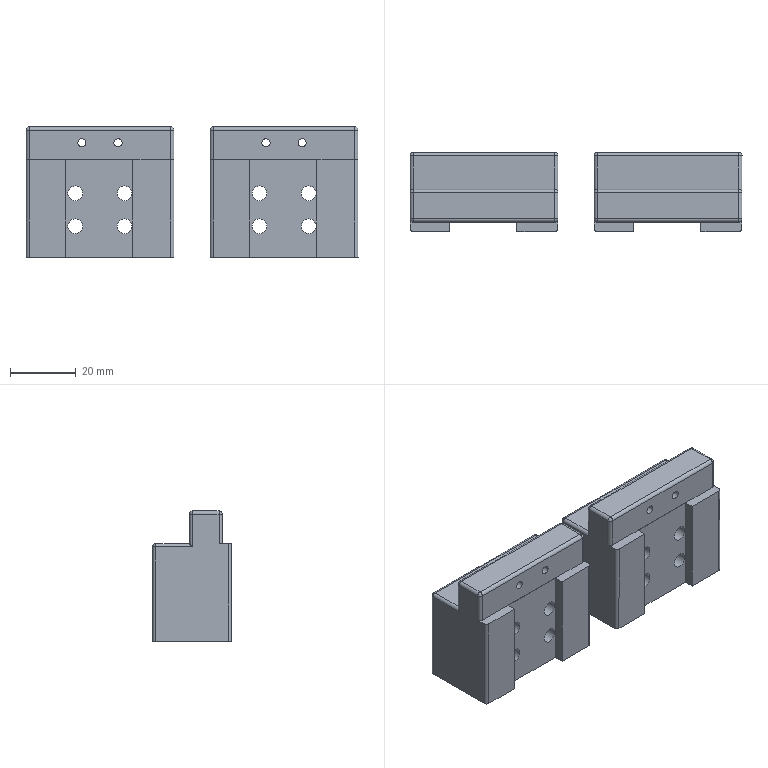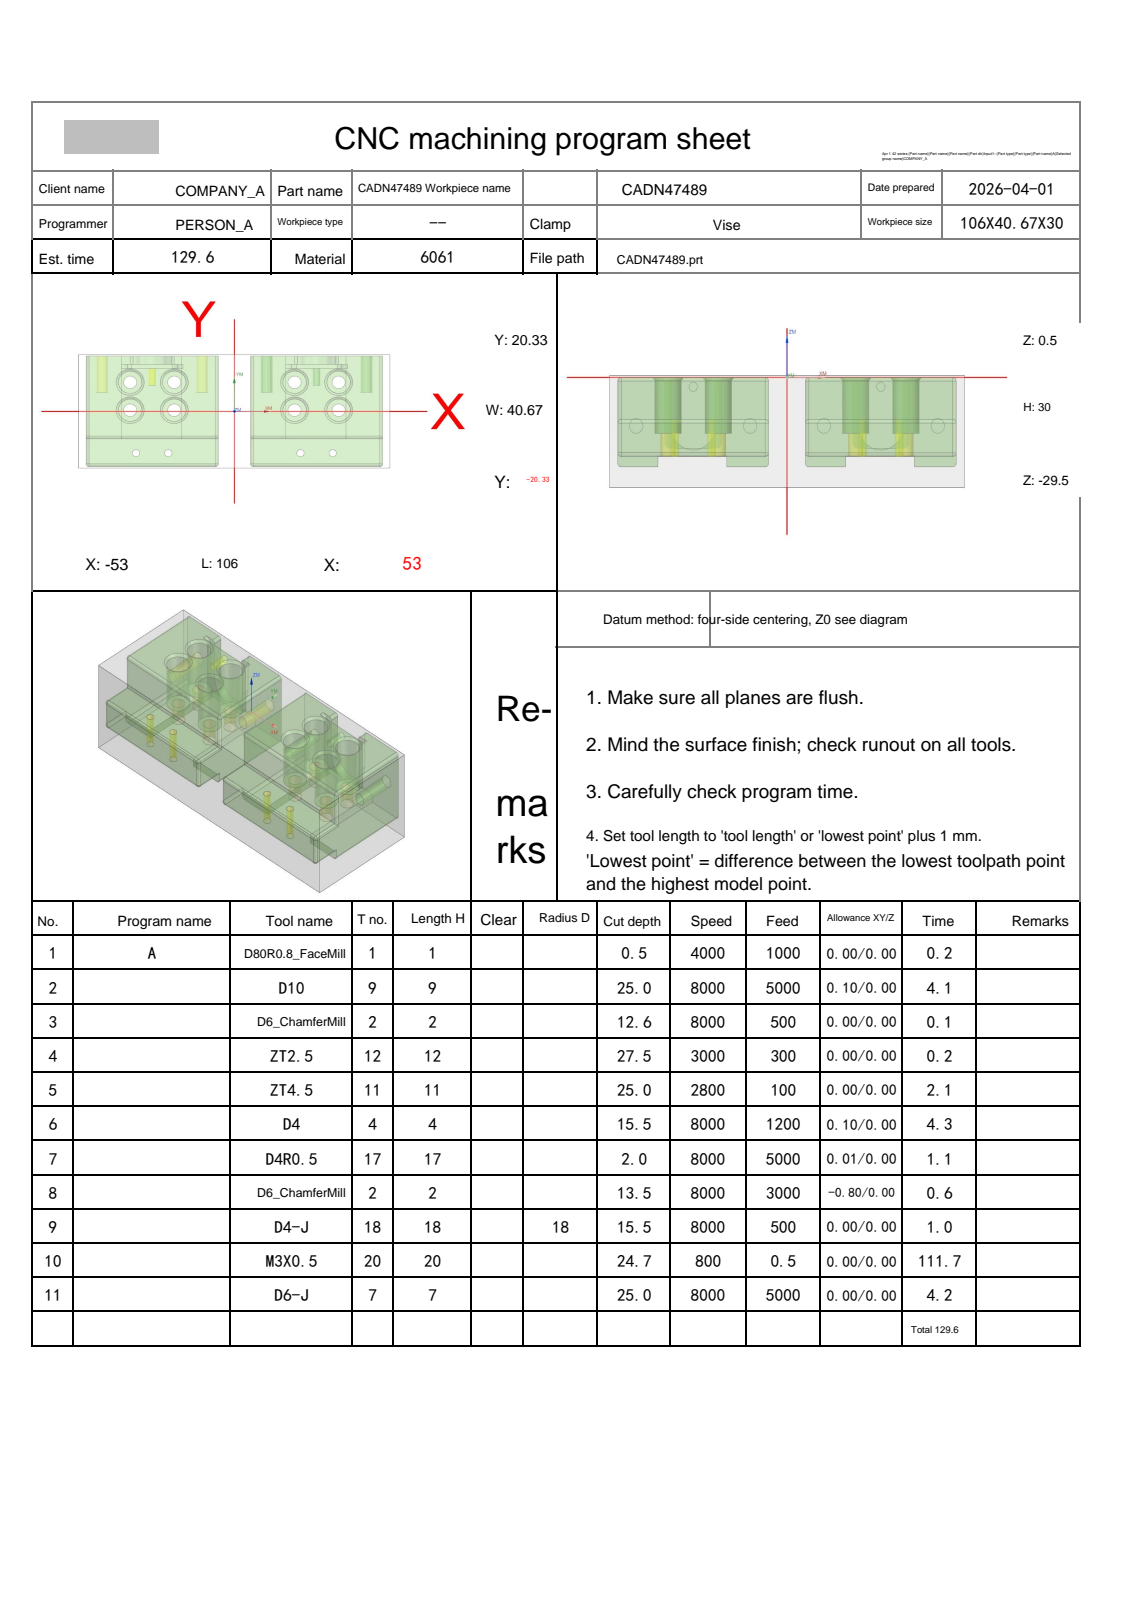NC program | NX | posted by the shop | part box 101.001 x 24.001 x 39.667 mm
Lines 1 to 2473 of 28944, first 1640 of 2471 lines:
%
O0001
(Machine time: 235.25 MIN)
(===Total Tool:10===)
(T1=D80R0.8 face mill D=80.  R=0.8  D-  H01 Z=0.    )
(T9=D10     D=10.  R=0.   D-  H09 Z=-24.5 )
(T2=D6_ChamferMill   D=6.   R=0.   D-  H02 Z=-13.01)
(T12=ZT2.5  D=2.5  DR_a=118 D-  H12 Z=-26.97)
(T11=ZT4.5  D=4.5  DR_a=118 D-  H11 Z=-24.45)
(T4=D4      D=4.   R=0.   D-  H04 Z=-15.  )
(T17=D4R0.5 D=4.   R=0.5  D-  H17 Z=-1.5  )
(T18=D4-J   D=4.   R=0.   D18 H18 Z=-15.  )
(T20=M3X0.5 D=2.5  DR_a=180 D-  H20 Z=-24.22)
(T7=D6-J    D=6.   R=0.   D7  H07 Z=-24.5 )
G80 G90 G17 G49 G40
G91 G28 Z0
M01
N1 T01 M06
(D80R0.8 face mill  D=80. R=0.8 H=01 ce=0.00 di=0.00)
G00 G90 G54 X95.501 Y0.0 M03 S4000
G43 H01 Z20.
M08
Z2.
G01 Z0.0 F1000.
X90.501
X-90.5
X-95.5
Z2.
G00 Z20.
G91 G28 Z0.0
M05
M09
G91 G28 Z0.0
M01
N2 T09 M06
(D10  D=10. R=0. H=09 ce=0.10 di=0.00)
G00 G90 G54 X-52.062 Y-24.399 M03 S8000
G43 H09 Z20.
M08
Z.5
G01 X-53.212 Y-23.713 Z.495 F5000.
X-54.216 Y-22.755 Z.489
X-54.985 Y-21.576 Z.484
X-55.467 Y-20.254 Z.478
X-55.6 Y-19.136 Z.474
Y19.833 Z.322
G02 X-50.5 Y24.933 Z.291 I5.1 J0.0
G01 X-6.498 Z.12
X-5.496 Y24.932 Z.116
G02 X-.4 Y19.832 Z.084 I-.004 J-5.1
G01 Y-18.833 Z-.066
G02 X-6.5 Y-24.932 Z-.103 I-6.1 J.001
G01 X-49.741 Z-.272
X-50.776 Y-24.828 Z-.276
X-52.05 Y-24.406 Z-.281
X-53.212 Y-23.713 Z-.286
X-54.216 Y-22.755 Z-.292
X-54.985 Y-21.576 Z-.297
X-55.467 Y-20.254 Z-.303
X-55.6 Y-19.136 Z-.307
Y19.833 Z-.459
G02 X-50.5 Y24.933 Z-.49 I5.1 J0.0
G01 X-6.498 Z-.662
X-5.496 Y24.932 Z-.666
G02 X-.4 Y19.832 Z-.697 I-.004 J-5.1
G01 Y-18.833 Z-.847
G02 X-6.5 Y-24.932 Z-.885 I-6.1 J.001
G01 X-49.741 Z-1.053
X-50.776 Y-24.828 Z-1.057
X-52.05 Y-24.406 Z-1.062
X-53.212 Y-23.713 Z-1.068
X-54.216 Y-22.755 Z-1.073
X-54.985 Y-21.576 Z-1.079
X-55.467 Y-20.254 Z-1.084
X-55.6 Y-19.136 Z-1.088
Y19.833 Z-1.24
G02 X-50.5 Y24.933 Z-1.272 I5.1 J0.0
G01 X-6.498 Z-1.443
X-5.496 Y24.932 Z-1.447
G02 X-.4 Y19.832 Z-1.478 I-.004 J-5.1
G01 Y-18.833 Z-1.629
G02 X-6.5 Y-24.932 Z-1.666 I-6.1 J.001
G01 X-49.741 Z-1.834
X-50.776 Y-24.828 Z-1.838
X-52.05 Y-24.406 Z-1.844
X-53.212 Y-23.713 Z-1.849
X-54.216 Y-22.755 Z-1.854
X-54.985 Y-21.576 Z-1.86
X-55.467 Y-20.254 Z-1.865
X-55.6 Y-19.136 Z-1.87
Y19.833 Z-2.022
G02 X-50.5 Y24.933 Z-2.053 I5.1 J0.0
G01 X-6.498 Z-2.224
X-5.496 Y24.932 Z-2.228
G02 X-.4 Y19.832 Z-2.259 I-.004 J-5.1
G01 Y-18.833 Z-2.41
G02 X-6.5 Y-24.932 Z-2.447 I-6.1 J.001
G01 X-49.741 Z-2.616
X-50.776 Y-24.828 Z-2.62
X-52.05 Y-24.406 Z-2.625
X-53.212 Y-23.713 Z-2.63
X-54.216 Y-22.755 Z-2.636
X-54.985 Y-21.576 Z-2.641
X-55.467 Y-20.254 Z-2.647
X-55.6 Y-19.136 Z-2.651
Y19.833 Z-2.803
G02 X-50.5 Y24.933 Z-2.834 I5.1 J0.0
G01 X-6.498 Z-3.005
X-5.496 Y24.932 Z-3.009
G02 X-.4 Y19.832 Z-3.041 I-.004 J-5.1
G01 Y-18.833 Z-3.191
G02 X-6.5 Y-24.932 Z-3.228 I-6.1 J.001
G01 X-49.741 Z-3.397
X-50.776 Y-24.828 Z-3.401
X-52.05 Y-24.406 Z-3.406
X-53.212 Y-23.713 Z-3.411
X-54.216 Y-22.755 Z-3.417
X-54.985 Y-21.576 Z-3.422
X-55.467 Y-20.254 Z-3.428
X-55.6 Y-19.136 Z-3.432
Y19.833 Z-3.584
G02 X-50.5 Y24.933 Z-3.615 I5.1 J0.0
G01 X-6.498 Z-3.787
X-5.496 Y24.932 Z-3.791
G02 X-.4 Y19.832 Z-3.822 I-.004 J-5.1
G01 Y-18.833 Z-3.972
G02 X-6.5 Y-24.932 Z-4.01 I-6.1 J.001
G01 X-49.741 Z-4.178
X-50.776 Y-24.828 Z-4.182
X-52.05 Y-24.406 Z-4.187
X-53.212 Y-23.713 Z-4.193
X-54.216 Y-22.755 Z-4.198
X-54.985 Y-21.576 Z-4.204
X-55.467 Y-20.254 Z-4.209
X-55.6 Y-19.136 Z-4.214
Y19.833 Z-4.365
G02 X-50.5 Y24.933 Z-4.397 I5.1 J0.0
G01 X-6.498 Z-4.568
X-5.496 Y24.932 Z-4.572
G02 X-.4 Y19.832 Z-4.603 I-.004 J-5.1
G01 Y-18.833 Z-4.754
G02 X-6.5 Y-24.932 Z-4.791 I-6.1 J.001
G01 X-49.741 Z-4.959
X-50.776 Y-24.828 Z-4.964
X-52.05 Y-24.406 Z-4.969
X-53.212 Y-23.713 Z-4.974
X-54.216 Y-22.755 Z-4.979
X-54.985 Y-21.576 Z-4.985
X-55.467 Y-20.254 Z-4.99
X-55.6 Y-19.136 Z-4.995
Y19.833 Z-5.147
G02 X-50.5 Y24.933 Z-5.178 I5.1 J0.0
G01 X-6.498 Z-5.349
X-5.496 Y24.932 Z-5.353
G02 X-.4 Y19.832 Z-5.384 I-.004 J-5.1
G01 Y-18.833 Z-5.535
G02 X-6.5 Y-24.932 Z-5.572 I-6.1 J.001
G01 X-49.741 Z-5.741
X-50.776 Y-24.828 Z-5.745
X-52.05 Y-24.406 Z-5.75
X-53.212 Y-23.713 Z-5.755
X-54.216 Y-22.755 Z-5.761
X-54.985 Y-21.576 Z-5.766
X-55.467 Y-20.254 Z-5.772
X-55.6 Y-19.136 Z-5.776
Y19.833 Z-5.928
G02 X-50.5 Y24.933 Z-5.959 I5.1 J0.0
G01 X-6.498 Z-6.13
X-5.496 Y24.932 Z-6.134
G02 X-.4 Y19.832 Z-6.166 I-.004 J-5.1
G01 Y-18.833 Z-6.316
G02 X-6.5 Y-24.932 Z-6.354 I-6.1 J.001
G01 X-49.741 Z-6.522
X-50.776 Y-24.828 Z-6.526
X-52.05 Y-24.406 Z-6.531
X-53.212 Y-23.713 Z-6.537
X-54.216 Y-22.755 Z-6.542
X-54.985 Y-21.576 Z-6.547
X-55.467 Y-20.254 Z-6.553
X-55.6 Y-19.136 Z-6.557
Y19.833 Z-6.709
G02 X-50.5 Y24.933 Z-6.74 I5.1 J0.0
G01 X-6.498 Z-6.912
X-5.496 Y24.932 Z-6.916
G02 X-.4 Y19.832 Z-6.947 I-.004 J-5.1
G01 Y-18.833 Z-7.097
G02 X-6.5 Y-24.932 Z-7.135 I-6.1 J.001
G01 X-49.741 Z-7.303
X-50.776 Y-24.828 Z-7.307
X-52.05 Y-24.406 Z-7.313
X-53.212 Y-23.713 Z-7.318
X-54.216 Y-22.755 Z-7.323
X-54.985 Y-21.576 Z-7.329
X-55.467 Y-20.254 Z-7.334
X-55.6 Y-19.136 Z-7.339
Y19.833 Z-7.49
G02 X-50.5 Y24.933 Z-7.522 I5.1 J0.0
G01 X-6.498 Z-7.693
X-5.496 Y24.932 Z-7.697
G02 X-.4 Y19.832 Z-7.728 I-.004 J-5.1
G01 Y-18.833 Z-7.879
G02 X-6.5 Y-24.932 Z-7.916 I-6.1 J.001
G01 X-49.741 Z-8.084
X-50.776 Y-24.828 Z-8.089
X-52.05 Y-24.406 Z-8.094
X-53.212 Y-23.713 Z-8.099
X-54.216 Y-22.755 Z-8.104
X-54.985 Y-21.576 Z-8.11
X-55.467 Y-20.254 Z-8.115
X-55.6 Y-19.136 Z-8.12
Y19.833 Z-8.272
G02 X-50.5 Y24.933 Z-8.303 I5.1 J0.0
G01 X-6.498 Z-8.474
X-5.496 Y24.932 Z-8.478
G02 X-.4 Y19.832 Z-8.509 I-.004 J-5.1
G01 Y-18.833 Z-8.66
G02 X-6.5 Y-24.932 Z-8.697 I-6.1 J.001
G01 X-49.741 Z-8.866
X-50.776 Y-24.828 Z-8.87
X-52.05 Y-24.406 Z-8.875
X-53.212 Y-23.713 Z-8.88
X-54.216 Y-22.755 Z-8.886
X-54.985 Y-21.576 Z-8.891
X-55.467 Y-20.254 Z-8.897
X-55.6 Y-19.136 Z-8.901
Y19.833 Z-9.053
G02 X-50.5 Y24.933 Z-9.084 I5.1 J0.0
G01 X-6.498 Z-9.255
X-5.496 Y24.932 Z-9.259
G02 X-.4 Y19.832 Z-9.291 I-.004 J-5.1
G01 Y-18.833 Z-9.441
G02 X-6.5 Y-24.932 Z-9.479 I-6.1 J.001
G01 X-49.741 Z-9.647
X-50.776 Y-24.828 Z-9.651
X-52.05 Y-24.406 Z-9.656
X-53.212 Y-23.713 Z-9.662
X-54.216 Y-22.755 Z-9.667
X-54.985 Y-21.576 Z-9.672
X-55.467 Y-20.254 Z-9.678
X-55.6 Y-19.136 Z-9.682
Y19.833 Z-9.834
G02 X-50.5 Y24.933 Z-9.865 I5.1 J0.0
G01 X-6.498 Z-10.037
X-5.496 Y24.932 Z-10.041
G02 X-.4 Y19.832 Z-10.072 I-.004 J-5.1
G01 Y-18.833 Z-10.222
G02 X-6.5 Y-24.932 Z-10.26 I-6.1 J.001
G01 X-49.741 Z-10.428
X-50.776 Y-24.828 Z-10.432
X-52.05 Y-24.406 Z-10.438
X-53.212 Y-23.713 Z-10.443
X-54.216 Y-22.755 Z-10.448
X-54.985 Y-21.576 Z-10.454
X-55.467 Y-20.254 Z-10.459
X-55.6 Y-19.136 Z-10.464
Y19.833 Z-10.615
G02 X-50.5 Y24.933 Z-10.647 I5.1 J0.0
G01 X-6.498 Z-10.818
X-5.496 Y24.932 Z-10.822
G02 X-.4 Y19.832 Z-10.853 I-.004 J-5.1
G01 Y-18.833 Z-11.004
G02 X-6.5 Y-24.932 Z-11.041 I-6.1 J.001
G01 X-49.741 Z-11.21
X-50.776 Y-24.828 Z-11.214
X-52.05 Y-24.406 Z-11.219
X-53.212 Y-23.713 Z-11.224
X-54.216 Y-22.755 Z-11.229
X-54.985 Y-21.576 Z-11.235
X-55.467 Y-20.254 Z-11.24
X-55.6 Y-19.136 Z-11.245
Y19.833 Z-11.397
G02 X-50.5 Y24.933 Z-11.428 I5.1 J0.0
G01 X-6.498 Z-11.599
X-5.496 Y24.932 Z-11.603
G02 X-.4 Y19.832 Z-11.634 I-.004 J-5.1
G01 Y-18.833 Z-11.785
G02 X-6.5 Y-24.932 Z-11.822 I-6.1 J.001
G01 X-49.741 Z-11.991
X-50.776 Y-24.828 Z-11.995
X-52.05 Y-24.406 Z-12.
X-53.212 Y-23.713 Z-12.005
X-54.216 Y-22.755 Z-12.011
X-54.985 Y-21.576 Z-12.016
X-55.467 Y-20.254 Z-12.022
X-55.6 Y-19.136 Z-12.026
Y19.833 Z-12.178
G02 X-50.5 Y24.933 Z-12.209 I5.1 J0.0
G01 X-6.498 Z-12.381
X-5.496 Y24.932 Z-12.384
G02 X-.4 Y19.832 Z-12.416 I-.004 J-5.1
G01 Y-18.833 Z-12.566
G02 X-6.5 Y-24.932 Z-12.604 I-6.1 J.001
G01 X-49.741 Z-12.772
X-50.776 Y-24.828 Z-12.776
X-52.05 Y-24.406 Z-12.781
X-53.212 Y-23.713 Z-12.787
X-54.216 Y-22.755 Z-12.792
X-54.985 Y-21.576 Z-12.797
X-55.467 Y-20.254 Z-12.803
X-55.6 Y-19.136 Z-12.807
Y19.833 Z-12.959
G02 X-50.5 Y24.933 Z-12.99 I5.1 J0.0
G01 X-6.498 Z-13.162
X-5.496 Y24.932 Z-13.166
G02 X-.4 Y19.832 Z-13.197 I-.004 J-5.1
G01 Y-18.833 Z-13.347
G02 X-6.5 Y-24.932 Z-13.385 I-6.1 J.001
G01 X-49.741 Z-13.553
X-50.776 Y-24.828 Z-13.557
X-52.05 Y-24.406 Z-13.563
X-53.212 Y-23.713 Z-13.568
X-54.216 Y-22.755 Z-13.573
X-54.985 Y-21.576 Z-13.579
X-55.467 Y-20.254 Z-13.584
X-55.6 Y-19.136 Z-13.589
Y19.833 Z-13.74
G02 X-50.5 Y24.933 Z-13.772 I5.1 J0.0
G01 X-6.498 Z-13.943
X-5.496 Y24.932 Z-13.947
G02 X-.4 Y19.832 Z-13.978 I-.004 J-5.1
G01 Y-18.833 Z-14.129
G02 X-6.5 Y-24.932 Z-14.166 I-6.1 J.001
G01 X-49.741 Z-14.335
X-50.776 Y-24.828 Z-14.339
X-52.05 Y-24.406 Z-14.344
X-53.212 Y-23.713 Z-14.349
X-54.216 Y-22.755 Z-14.354
X-54.985 Y-21.576 Z-14.36
X-55.467 Y-20.254 Z-14.365
X-55.6 Y-19.136 Z-14.37
Y19.833 Z-14.522
G02 X-50.5 Y24.933 Z-14.553 I5.1 J0.0
G01 X-6.498 Z-14.724
X-5.496 Y24.932 Z-14.728
G02 X-.4 Y19.832 Z-14.759 I-.004 J-5.1
G01 Y-18.833 Z-14.91
G02 X-6.5 Y-24.932 Z-14.947 I-6.1 J.001
G01 X-49.741 Z-15.116
X-50.776 Y-24.828 Z-15.12
X-52.05 Y-24.406 Z-15.125
X-53.212 Y-23.713 Z-15.13
X-54.216 Y-22.755 Z-15.136
X-54.985 Y-21.576 Z-15.141
X-55.467 Y-20.254 Z-15.147
X-55.6 Y-19.136 Z-15.151
Y19.833 Z-15.303
G02 X-50.5 Y24.933 Z-15.334 I5.1 J0.0
G01 X-6.498 Z-15.506
X-5.496 Y24.932 Z-15.509
G02 X-.4 Y19.832 Z-15.541 I-.004 J-5.1
G01 Y-18.833 Z-15.691
G02 X-6.5 Y-24.932 Z-15.729 I-6.1 J.001
G01 X-49.741 Z-15.897
X-50.776 Y-24.828 Z-15.901
X-52.05 Y-24.406 Z-15.906
X-53.212 Y-23.713 Z-15.912
X-54.216 Y-22.755 Z-15.917
X-54.985 Y-21.576 Z-15.922
X-55.467 Y-20.254 Z-15.928
X-55.6 Y-19.136 Z-15.932
Y19.833 Z-16.084
G02 X-50.5 Y24.933 Z-16.115 I5.1 J0.0
G01 X-6.498 Z-16.287
X-5.496 Y24.932 Z-16.291
G02 X-.4 Y19.832 Z-16.322 I-.004 J-5.1
G01 Y-18.833 Z-16.473
G02 X-6.5 Y-24.932 Z-16.51 I-6.1 J.001
G01 X-49.741 Z-16.678
X-50.776 Y-24.828 Z-16.682
X-52.05 Y-24.406 Z-16.688
X-53.212 Y-23.713 Z-16.693
X-54.216 Y-22.755 Z-16.698
X-54.985 Y-21.576 Z-16.704
X-55.467 Y-20.254 Z-16.709
X-55.6 Y-19.136 Z-16.714
Y19.833 Z-16.865
G02 X-50.5 Y24.933 Z-16.897 I5.1 J0.0
G01 X-6.498 Z-17.068
X-5.496 Y24.932 Z-17.072
G02 X-.4 Y19.832 Z-17.103 I-.004 J-5.1
G01 Y-18.833 Z-17.254
G02 X-6.5 Y-24.932 Z-17.291 I-6.1 J.001
G01 X-49.741 Z-17.46
X-50.776 Y-24.828 Z-17.464
X-52.05 Y-24.406 Z-17.469
X-53.212 Y-23.713 Z-17.474
X-54.216 Y-22.755 Z-17.48
X-54.985 Y-21.576 Z-17.485
X-55.467 Y-20.254 Z-17.49
X-55.6 Y-19.136 Z-17.495
Y19.833 Z-17.647
G02 X-50.5 Y24.933 Z-17.678 I5.1 J0.0
G01 X-6.498 Z-17.849
X-5.496 Y24.932 Z-17.853
G02 X-.4 Y19.832 Z-17.884 I-.004 J-5.1
G01 Y-18.833 Z-18.035
G02 X-6.5 Y-24.932 Z-18.072 I-6.1 J.001
G01 X-49.741 Z-18.241
X-50.776 Y-24.828 Z-18.245
X-52.05 Y-24.406 Z-18.25
X-53.212 Y-23.713 Z-18.255
X-54.216 Y-22.755 Z-18.261
X-54.985 Y-21.576 Z-18.266
X-55.467 Y-20.254 Z-18.272
X-55.6 Y-19.136 Z-18.276
Y19.833 Z-18.428
G02 X-50.5 Y24.933 Z-18.459 I5.1 J0.0
G01 X-6.498 Z-18.631
X-5.496 Y24.932 Z-18.634
G02 X-.4 Y19.832 Z-18.666 I-.004 J-5.1
G01 Y-18.833 Z-18.816
G02 X-6.5 Y-24.932 Z-18.854 I-6.1 J.001
G01 X-49.741 Z-19.022
X-50.776 Y-24.828 Z-19.026
X-52.05 Y-24.406 Z-19.031
X-53.212 Y-23.713 Z-19.037
X-54.216 Y-22.755 Z-19.042
X-54.985 Y-21.576 Z-19.047
X-55.467 Y-20.254 Z-19.053
X-55.6 Y-19.136 Z-19.057
Y19.833 Z-19.209
G02 X-50.5 Y24.933 Z-19.24 I5.1 J0.0
G01 X-6.498 Z-19.412
X-5.496 Y24.932 Z-19.416
G02 X-.4 Y19.832 Z-19.447 I-.004 J-5.1
G01 Y-18.833 Z-19.598
G02 X-6.5 Y-24.932 Z-19.635 I-6.1 J.001
G01 X-49.741 Z-19.803
X-50.776 Y-24.828 Z-19.807
X-52.05 Y-24.406 Z-19.813
X-53.212 Y-23.713 Z-19.818
X-54.216 Y-22.755 Z-19.823
X-54.985 Y-21.576 Z-19.829
X-55.467 Y-20.254 Z-19.834
X-55.6 Y-19.136 Z-19.839
Y19.833 Z-19.99
G02 X-50.5 Y24.933 Z-20.022 I5.1 J0.0
G01 X-6.498 Z-20.193
X-5.496 Y24.932 Z-20.197
G02 X-.4 Y19.832 Z-20.228 I-.004 J-5.1
G01 Y-18.833 Z-20.379
G02 X-6.5 Y-24.932 Z-20.416 I-6.1 J.001
G01 X-49.741 Z-20.585
X-50.776 Y-24.828 Z-20.589
X-52.05 Y-24.406 Z-20.594
X-53.212 Y-23.713 Z-20.599
X-54.216 Y-22.755 Z-20.605
X-54.985 Y-21.576 Z-20.61
X-55.467 Y-20.254 Z-20.615
X-55.6 Y-19.136 Z-20.62
Y19.833 Z-20.772
G02 X-50.5 Y24.933 Z-20.803 I5.1 J0.0
G01 X-6.498 Z-20.974
X-5.496 Y24.932 Z-20.978
G02 X-.4 Y19.832 Z-21.009 I-.004 J-5.1
G01 Y-18.833 Z-21.16
G02 X-6.5 Y-24.932 Z-21.197 I-6.1 J.001
G01 X-49.741 Z-21.366
X-50.776 Y-24.828 Z-21.37
X-52.05 Y-24.406 Z-21.375
X-53.212 Y-23.713 Z-21.38
X-54.216 Y-22.755 Z-21.386
X-54.985 Y-21.576 Z-21.391
X-55.467 Y-20.254 Z-21.397
X-55.6 Y-19.136 Z-21.401
Y19.833 Z-21.553
G02 X-50.5 Y24.933 Z-21.584 I5.1 J0.0
G01 X-6.498 Z-21.756
X-5.496 Y24.932 Z-21.759
G02 X-.4 Y19.832 Z-21.791 I-.004 J-5.1
G01 Y-18.833 Z-21.941
G02 X-6.5 Y-24.932 Z-21.979 I-6.1 J.001
G01 X-49.741 Z-22.147
X-50.776 Y-24.828 Z-22.151
X-52.05 Y-24.406 Z-22.156
X-53.212 Y-23.713 Z-22.162
X-54.216 Y-22.755 Z-22.167
X-54.985 Y-21.576 Z-22.173
X-55.467 Y-20.254 Z-22.178
X-55.6 Y-19.136 Z-22.182
Y19.833 Z-22.334
G02 X-50.5 Y24.933 Z-22.365 I5.1 J0.0
G01 X-6.498 Z-22.537
X-5.496 Y24.932 Z-22.541
G02 X-.4 Y19.832 Z-22.572 I-.004 J-5.1
G01 Y-18.833 Z-22.723
G02 X-6.5 Y-24.932 Z-22.76 I-6.1 J.001
G01 X-49.741 Z-22.928
X-50.776 Y-24.828 Z-22.932
X-52.05 Y-24.406 Z-22.938
X-53.212 Y-23.713 Z-22.943
X-54.216 Y-22.755 Z-22.948
X-54.985 Y-21.576 Z-22.954
X-55.467 Y-20.254 Z-22.959
X-55.6 Y-19.136 Z-22.964
Y19.833 Z-23.115
G02 X-50.5 Y24.933 Z-23.147 I5.1 J0.0
G01 X-6.498 Z-23.318
X-5.496 Y24.932 Z-23.322
G02 X-.4 Y19.832 Z-23.353 I-.004 J-5.1
G01 Y-18.833 Z-23.504
G02 X-6.5 Y-24.932 Z-23.541 I-6.1 J.001
G01 X-49.741 Z-23.71
X-50.776 Y-24.828 Z-23.714
X-52.05 Y-24.406 Z-23.719
X-53.212 Y-23.713 Z-23.724
X-54.216 Y-22.755 Z-23.73
X-54.985 Y-21.576 Z-23.735
X-55.467 Y-20.254 Z-23.741
X-55.6 Y-19.136 Z-23.745
Y19.833 Z-23.897
G02 X-50.5 Y24.933 Z-23.928 I5.1 J0.0
G01 X-6.498 Z-24.099
X-5.496 Y24.932 Z-24.103
G02 X-.4 Y19.832 Z-24.134 I-.004 J-5.1
G01 Y-18.833 Z-24.285
G02 X-6.5 Y-24.932 Z-24.322 I-6.1 J.001
G01 X-49.741 Z-24.491
X-50.776 Y-24.828 Z-24.495
X-52.05 Y-24.406 Z-24.5
X-53.212 Y-23.713
X-54.216 Y-22.755
X-54.985 Y-21.576
X-55.467 Y-20.254
X-55.6 Y-19.136
Y19.833
G02 X-50.5 Y24.933 I5.1 J0.0
G01 X-6.498
X-5.496 Y24.932
G02 X-.4 Y19.832 I-.004 J-5.1
G01 Y-18.833
G02 X-6.5 Y-24.932 I-6.1 J.001
G01 X-49.741
X-50.776 Y-24.828
X-52.05 Y-24.406
X-52.062 Y-24.399
X-52.491 Y-24.143
Z-23.5
G00 Z20.
X3.938 Y-24.4
Z.5
G01 X2.788 Y-23.714 Z.495
X1.784 Y-22.756 Z.489
X1.015 Y-21.577 Z.484
X.533 Y-20.255 Z.478
X.4 Y-19.137 Z.474
Y19.832 Z.322
G02 X5.5 Y24.932 Z.291 I5.1 J0.0
G01 X49.502 Z.12
X50.504 Y24.931 Z.116
G02 X55.6 Y19.831 Z.084 I-.004 J-5.1
G01 Y-18.834 Z-.066
G02 X49.5 Y-24.933 Z-.103 I-6.1 J.001
G01 X6.259 Z-.272
X5.224 Y-24.829 Z-.276
X3.95 Y-24.406 Z-.281
X2.788 Y-23.714 Z-.286
X1.784 Y-22.756 Z-.292
X1.015 Y-21.577 Z-.297
X.533 Y-20.255 Z-.303
X.4 Y-19.137 Z-.307
Y19.832 Z-.459
G02 X5.5 Y24.932 Z-.49 I5.1 J0.0
G01 X49.502 Z-.662
X50.504 Y24.931 Z-.666
G02 X55.6 Y19.831 Z-.697 I-.004 J-5.1
G01 Y-18.834 Z-.847
G02 X49.5 Y-24.933 Z-.885 I-6.1 J.001
G01 X6.259 Z-1.053
X5.224 Y-24.829 Z-1.057
X3.95 Y-24.406 Z-1.062
X2.788 Y-23.714 Z-1.068
X1.784 Y-22.756 Z-1.073
X1.015 Y-21.577 Z-1.079
X.533 Y-20.255 Z-1.084
X.4 Y-19.137 Z-1.088
Y19.832 Z-1.24
G02 X5.5 Y24.932 Z-1.272 I5.1 J0.0
G01 X49.502 Z-1.443
X50.504 Y24.931 Z-1.447
G02 X55.6 Y19.831 Z-1.478 I-.004 J-5.1
G01 Y-18.834 Z-1.629
G02 X49.5 Y-24.933 Z-1.666 I-6.1 J.001
G01 X6.259 Z-1.834
X5.224 Y-24.829 Z-1.838
X3.95 Y-24.406 Z-1.844
X2.788 Y-23.714 Z-1.849
X1.784 Y-22.756 Z-1.854
X1.015 Y-21.577 Z-1.86
X.533 Y-20.255 Z-1.865
X.4 Y-19.137 Z-1.87
Y19.832 Z-2.022
G02 X5.5 Y24.932 Z-2.053 I5.1 J0.0
G01 X49.502 Z-2.224
X50.504 Y24.931 Z-2.228
G02 X55.6 Y19.831 Z-2.259 I-.004 J-5.1
G01 Y-18.834 Z-2.41
G02 X49.5 Y-24.933 Z-2.447 I-6.1 J.001
G01 X6.259 Z-2.616
X5.224 Y-24.829 Z-2.62
X3.95 Y-24.406 Z-2.625
X2.788 Y-23.714 Z-2.63
X1.784 Y-22.756 Z-2.636
X1.015 Y-21.577 Z-2.641
X.533 Y-20.255 Z-2.647
X.4 Y-19.137 Z-2.651
Y19.832 Z-2.803
G02 X5.5 Y24.932 Z-2.834 I5.1 J0.0
G01 X49.502 Z-3.005
X50.504 Y24.931 Z-3.009
G02 X55.6 Y19.831 Z-3.041 I-.004 J-5.1
G01 Y-18.834 Z-3.191
G02 X49.5 Y-24.933 Z-3.228 I-6.1 J.001
G01 X6.259 Z-3.397
X5.224 Y-24.829 Z-3.401
X3.95 Y-24.406 Z-3.406
X2.788 Y-23.714 Z-3.411
X1.784 Y-22.756 Z-3.417
X1.015 Y-21.577 Z-3.422
X.533 Y-20.255 Z-3.428
X.4 Y-19.137 Z-3.432
Y19.832 Z-3.584
G02 X5.5 Y24.932 Z-3.615 I5.1 J0.0
G01 X49.502 Z-3.787
X50.504 Y24.931 Z-3.791
G02 X55.6 Y19.831 Z-3.822 I-.004 J-5.1
G01 Y-18.834 Z-3.972
G02 X49.5 Y-24.933 Z-4.01 I-6.1 J.001
G01 X6.259 Z-4.178
X5.224 Y-24.829 Z-4.182
X3.95 Y-24.406 Z-4.187
X2.788 Y-23.714 Z-4.193
X1.784 Y-22.756 Z-4.198
X1.015 Y-21.577 Z-4.204
X.533 Y-20.255 Z-4.209
X.4 Y-19.137 Z-4.214
Y19.832 Z-4.365
G02 X5.5 Y24.932 Z-4.397 I5.1 J0.0
G01 X49.502 Z-4.568
X50.504 Y24.931 Z-4.572
G02 X55.6 Y19.831 Z-4.603 I-.004 J-5.1
G01 Y-18.834 Z-4.754
G02 X49.5 Y-24.933 Z-4.791 I-6.1 J.001
G01 X6.259 Z-4.959
X5.224 Y-24.829 Z-4.964
X3.95 Y-24.406 Z-4.969
X2.788 Y-23.714 Z-4.974
X1.784 Y-22.756 Z-4.979
X1.015 Y-21.577 Z-4.985
X.533 Y-20.255 Z-4.99
X.4 Y-19.137 Z-4.995
Y19.832 Z-5.147
G02 X5.5 Y24.932 Z-5.178 I5.1 J0.0
G01 X49.502 Z-5.349
X50.504 Y24.931 Z-5.353
G02 X55.6 Y19.831 Z-5.384 I-.004 J-5.1
G01 Y-18.834 Z-5.535
G02 X49.5 Y-24.933 Z-5.572 I-6.1 J.001
G01 X6.259 Z-5.741
X5.224 Y-24.829 Z-5.745
X3.95 Y-24.406 Z-5.75
X2.788 Y-23.714 Z-5.755
X1.784 Y-22.756 Z-5.761
X1.015 Y-21.577 Z-5.766
X.533 Y-20.255 Z-5.772
X.4 Y-19.137 Z-5.776
Y19.832 Z-5.928
G02 X5.5 Y24.932 Z-5.959 I5.1 J0.0
G01 X49.502 Z-6.13
X50.504 Y24.931 Z-6.134
G02 X55.6 Y19.831 Z-6.166 I-.004 J-5.1
G01 Y-18.834 Z-6.316
G02 X49.5 Y-24.933 Z-6.354 I-6.1 J.001
G01 X6.259 Z-6.522
X5.224 Y-24.829 Z-6.526
X3.95 Y-24.406 Z-6.531
X2.788 Y-23.714 Z-6.537
X1.784 Y-22.756 Z-6.542
X1.015 Y-21.577 Z-6.547
X.533 Y-20.255 Z-6.553
X.4 Y-19.137 Z-6.557
Y19.832 Z-6.709
G02 X5.5 Y24.932 Z-6.74 I5.1 J0.0
G01 X49.502 Z-6.912
X50.504 Y24.931 Z-6.916
G02 X55.6 Y19.831 Z-6.947 I-.004 J-5.1
G01 Y-18.834 Z-7.097
G02 X49.5 Y-24.933 Z-7.135 I-6.1 J.001
G01 X6.259 Z-7.303
X5.224 Y-24.829 Z-7.307
X3.95 Y-24.406 Z-7.313
X2.788 Y-23.714 Z-7.318
X1.784 Y-22.756 Z-7.323
X1.015 Y-21.577 Z-7.329
X.533 Y-20.255 Z-7.334
X.4 Y-19.137 Z-7.339
Y19.832 Z-7.49
G02 X5.5 Y24.932 Z-7.522 I5.1 J0.0
G01 X49.502 Z-7.693
X50.504 Y24.931 Z-7.697
G02 X55.6 Y19.831 Z-7.728 I-.004 J-5.1
G01 Y-18.834 Z-7.879
G02 X49.5 Y-24.933 Z-7.916 I-6.1 J.001
G01 X6.259 Z-8.084
X5.224 Y-24.829 Z-8.089
X3.95 Y-24.406 Z-8.094
X2.788 Y-23.714 Z-8.099
X1.784 Y-22.756 Z-8.104
X1.015 Y-21.577 Z-8.11
X.533 Y-20.255 Z-8.115
X.4 Y-19.137 Z-8.12
Y19.832 Z-8.272
G02 X5.5 Y24.932 Z-8.303 I5.1 J0.0
G01 X49.502 Z-8.474
X50.504 Y24.931 Z-8.478
G02 X55.6 Y19.831 Z-8.509 I-.004 J-5.1
G01 Y-18.834 Z-8.66
G02 X49.5 Y-24.933 Z-8.697 I-6.1 J.001
G01 X6.259 Z-8.866
X5.224 Y-24.829 Z-8.87
X3.95 Y-24.406 Z-8.875
X2.788 Y-23.714 Z-8.88
X1.784 Y-22.756 Z-8.886
X1.015 Y-21.577 Z-8.891
X.533 Y-20.255 Z-8.897
X.4 Y-19.137 Z-8.901
Y19.832 Z-9.053
G02 X5.5 Y24.932 Z-9.084 I5.1 J0.0
G01 X49.502 Z-9.255
X50.504 Y24.931 Z-9.259
G02 X55.6 Y19.831 Z-9.291 I-.004 J-5.1
G01 Y-18.834 Z-9.441
G02 X49.5 Y-24.933 Z-9.479 I-6.1 J.001
G01 X6.259 Z-9.647
X5.224 Y-24.829 Z-9.651
X3.95 Y-24.406 Z-9.656
X2.788 Y-23.714 Z-9.662
X1.784 Y-22.756 Z-9.667
X1.015 Y-21.577 Z-9.672
X.533 Y-20.255 Z-9.678
X.4 Y-19.137 Z-9.682
Y19.832 Z-9.834
G02 X5.5 Y24.932 Z-9.865 I5.1 J0.0
G01 X49.502 Z-10.037
X50.504 Y24.931 Z-10.041
G02 X55.6 Y19.831 Z-10.072 I-.004 J-5.1
G01 Y-18.834 Z-10.222
G02 X49.5 Y-24.933 Z-10.26 I-6.1 J.001
G01 X6.259 Z-10.428
X5.224 Y-24.829 Z-10.432
X3.95 Y-24.406 Z-10.438
X2.788 Y-23.714 Z-10.443
X1.784 Y-22.756 Z-10.448
X1.015 Y-21.577 Z-10.454
X.533 Y-20.255 Z-10.459
X.4 Y-19.137 Z-10.464
Y19.832 Z-10.615
G02 X5.5 Y24.932 Z-10.647 I5.1 J0.0
G01 X49.502 Z-10.818
X50.504 Y24.931 Z-10.822
G02 X55.6 Y19.831 Z-10.853 I-.004 J-5.1
G01 Y-18.834 Z-11.004
G02 X49.5 Y-24.933 Z-11.041 I-6.1 J.001
G01 X6.259 Z-11.21
X5.224 Y-24.829 Z-11.214
X3.95 Y-24.406 Z-11.219
X2.788 Y-23.714 Z-11.224
X1.784 Y-22.756 Z-11.229
X1.015 Y-21.577 Z-11.235
X.533 Y-20.255 Z-11.24
X.4 Y-19.137 Z-11.245
Y19.832 Z-11.397
G02 X5.5 Y24.932 Z-11.428 I5.1 J0.0
G01 X49.502 Z-11.599
X50.504 Y24.931 Z-11.603
G02 X55.6 Y19.831 Z-11.634 I-.004 J-5.1
G01 Y-18.834 Z-11.785
G02 X49.5 Y-24.933 Z-11.822 I-6.1 J.001
G01 X6.259 Z-11.991
X5.224 Y-24.829 Z-11.995
X3.95 Y-24.406 Z-12.
X2.788 Y-23.714 Z-12.005
X1.784 Y-22.756 Z-12.011
X1.015 Y-21.577 Z-12.016
X.533 Y-20.255 Z-12.022
X.4 Y-19.137 Z-12.026
Y19.832 Z-12.178
G02 X5.5 Y24.932 Z-12.209 I5.1 J0.0
G01 X49.502 Z-12.381
X50.504 Y24.931 Z-12.384
G02 X55.6 Y19.831 Z-12.416 I-.004 J-5.1
G01 Y-18.834 Z-12.566
G02 X49.5 Y-24.933 Z-12.604 I-6.1 J.001
G01 X6.259 Z-12.772
X5.224 Y-24.829 Z-12.776
X3.95 Y-24.406 Z-12.781
X2.788 Y-23.714 Z-12.787
X1.784 Y-22.756 Z-12.792
X1.015 Y-21.577 Z-12.797
X.533 Y-20.255 Z-12.803
X.4 Y-19.137 Z-12.807
Y19.832 Z-12.959
G02 X5.5 Y24.932 Z-12.99 I5.1 J0.0
G01 X49.502 Z-13.162
X50.504 Y24.931 Z-13.166
G02 X55.6 Y19.831 Z-13.197 I-.004 J-5.1
G01 Y-18.834 Z-13.347
G02 X49.5 Y-24.933 Z-13.385 I-6.1 J.001
G01 X6.259 Z-13.553
X5.224 Y-24.829 Z-13.557
X3.95 Y-24.406 Z-13.563
X2.788 Y-23.714 Z-13.568
X1.784 Y-22.756 Z-13.573
X1.015 Y-21.577 Z-13.579
X.533 Y-20.255 Z-13.584
X.4 Y-19.137 Z-13.589
Y19.832 Z-13.74
G02 X5.5 Y24.932 Z-13.772 I5.1 J0.0
G01 X49.502 Z-13.943
X50.504 Y24.931 Z-13.947
G02 X55.6 Y19.831 Z-13.978 I-.004 J-5.1
G01 Y-18.834 Z-14.129
G02 X49.5 Y-24.933 Z-14.166 I-6.1 J.001
G01 X6.259 Z-14.335
X5.224 Y-24.829 Z-14.339
X3.95 Y-24.406 Z-14.344
X2.788 Y-23.714 Z-14.349
X1.784 Y-22.756 Z-14.354
X1.015 Y-21.577 Z-14.36
X.533 Y-20.255 Z-14.365
X.4 Y-19.137 Z-14.37
Y19.832 Z-14.522
G02 X5.5 Y24.932 Z-14.553 I5.1 J0.0
G01 X49.502 Z-14.724
X50.504 Y24.931 Z-14.728
G02 X55.6 Y19.831 Z-14.759 I-.004 J-5.1
G01 Y-18.834 Z-14.91
G02 X49.5 Y-24.933 Z-14.947 I-6.1 J.001
G01 X6.259 Z-15.116
X5.224 Y-24.829 Z-15.12
X3.95 Y-24.406 Z-15.125
X2.788 Y-23.714 Z-15.13
X1.784 Y-22.756 Z-15.136
X1.015 Y-21.577 Z-15.141
X.533 Y-20.255 Z-15.147
X.4 Y-19.137 Z-15.151
Y19.832 Z-15.303
G02 X5.5 Y24.932 Z-15.334 I5.1 J0.0
G01 X49.502 Z-15.506
X50.504 Y24.931 Z-15.509
G02 X55.6 Y19.831 Z-15.541 I-.004 J-5.1
G01 Y-18.834 Z-15.691
G02 X49.5 Y-24.933 Z-15.729 I-6.1 J.001
G01 X6.259 Z-15.897
X5.224 Y-24.829 Z-15.901
X3.95 Y-24.406 Z-15.906
X2.788 Y-23.714 Z-15.912
X1.784 Y-22.756 Z-15.917
X1.015 Y-21.577 Z-15.922
X.533 Y-20.255 Z-15.928
X.4 Y-19.137 Z-15.932
Y19.832 Z-16.084
G02 X5.5 Y24.932 Z-16.115 I5.1 J0.0
G01 X49.502 Z-16.287
X50.504 Y24.931 Z-16.291
G02 X55.6 Y19.831 Z-16.322 I-.004 J-5.1
G01 Y-18.834 Z-16.473
G02 X49.5 Y-24.933 Z-16.51 I-6.1 J.001
G01 X6.259 Z-16.678
X5.224 Y-24.829 Z-16.682
X3.95 Y-24.406 Z-16.688
X2.788 Y-23.714 Z-16.693
X1.784 Y-22.756 Z-16.698
X1.015 Y-21.577 Z-16.704
X.533 Y-20.255 Z-16.709
X.4 Y-19.137 Z-16.714
Y19.832 Z-16.865
G02 X5.5 Y24.932 Z-16.897 I5.1 J0.0
G01 X49.502 Z-17.068
X50.504 Y24.931 Z-17.072
G02 X55.6 Y19.831 Z-17.103 I-.004 J-5.1
G01 Y-18.834 Z-17.254
G02 X49.5 Y-24.933 Z-17.291 I-6.1 J.001
G01 X6.259 Z-17.46
X5.224 Y-24.829 Z-17.464
X3.95 Y-24.406 Z-17.469
X2.788 Y-23.714 Z-17.474
X1.784 Y-22.756 Z-17.48
X1.015 Y-21.577 Z-17.485
X.533 Y-20.255 Z-17.49
X.4 Y-19.137 Z-17.495
Y19.832 Z-17.647
G02 X5.5 Y24.932 Z-17.678 I5.1 J0.0
G01 X49.502 Z-17.849
X50.504 Y24.931 Z-17.853
G02 X55.6 Y19.831 Z-17.884 I-.004 J-5.1
G01 Y-18.834 Z-18.035
G02 X49.5 Y-24.933 Z-18.072 I-6.1 J.001
G01 X6.259 Z-18.241
X5.224 Y-24.829 Z-18.245
X3.95 Y-24.406 Z-18.25
X2.788 Y-23.714 Z-18.255
X1.784 Y-22.756 Z-18.261
X1.015 Y-21.577 Z-18.266
X.533 Y-20.255 Z-18.272
X.4 Y-19.137 Z-18.276
Y19.832 Z-18.428
G02 X5.5 Y24.932 Z-18.459 I5.1 J0.0
G01 X49.502 Z-18.631
X50.504 Y24.931 Z-18.634
G02 X55.6 Y19.831 Z-18.666 I-.004 J-5.1
G01 Y-18.834 Z-18.816
G02 X49.5 Y-24.933 Z-18.854 I-6.1 J.001
G01 X6.259 Z-19.022
X5.224 Y-24.829 Z-19.026
X3.95 Y-24.406 Z-19.031
X2.788 Y-23.714 Z-19.037
X1.784 Y-22.756 Z-19.042
X1.015 Y-21.577 Z-19.047
X.533 Y-20.255 Z-19.053
X.4 Y-19.137 Z-19.057
Y19.832 Z-19.209
G02 X5.5 Y24.932 Z-19.24 I5.1 J0.0
G01 X49.502 Z-19.412
X50.504 Y24.931 Z-19.416
G02 X55.6 Y19.831 Z-19.447 I-.004 J-5.1
G01 Y-18.834 Z-19.598
G02 X49.5 Y-24.933 Z-19.635 I-6.1 J.001
G01 X6.259 Z-19.803
X5.224 Y-24.829 Z-19.807
X3.95 Y-24.406 Z-19.813
X2.788 Y-23.714 Z-19.818
X1.784 Y-22.756 Z-19.823
X1.015 Y-21.577 Z-19.829
X.533 Y-20.255 Z-19.834
X.4 Y-19.137 Z-19.839
Y19.832 Z-19.99
G02 X5.5 Y24.932 Z-20.022 I5.1 J0.0
G01 X49.502 Z-20.193
X50.504 Y24.931 Z-20.197
G02 X55.6 Y19.831 Z-20.228 I-.004 J-5.1
G01 Y-18.834 Z-20.379
G02 X49.5 Y-24.933 Z-20.416 I-6.1 J.001
G01 X6.259 Z-20.585
X5.224 Y-24.829 Z-20.589
X3.95 Y-24.406 Z-20.594
X2.788 Y-23.714 Z-20.599
X1.784 Y-22.756 Z-20.605
X1.015 Y-21.577 Z-20.61
X.533 Y-20.255 Z-20.615
X.4 Y-19.137 Z-20.62
Y19.832 Z-20.772
G02 X5.5 Y24.932 Z-20.803 I5.1 J0.0
G01 X49.502 Z-20.974
X50.504 Y24.931 Z-20.978
G02 X55.6 Y19.831 Z-21.009 I-.004 J-5.1
G01 Y-18.834 Z-21.16
G02 X49.5 Y-24.933 Z-21.197 I-6.1 J.001
G01 X6.259 Z-21.366
X5.224 Y-24.829 Z-21.37
X3.95 Y-24.406 Z-21.375
X2.788 Y-23.714 Z-21.38
X1.784 Y-22.756 Z-21.386
X1.015 Y-21.577 Z-21.391
X.533 Y-20.255 Z-21.397
X.4 Y-19.137 Z-21.401
Y19.832 Z-21.553
G02 X5.5 Y24.932 Z-21.584 I5.1 J0.0
G01 X49.502 Z-21.756
X50.504 Y24.931 Z-21.759
G02 X55.6 Y19.831 Z-21.791 I-.004 J-5.1
G01 Y-18.834 Z-21.941
G02 X49.5 Y-24.933 Z-21.979 I-6.1 J.001
G01 X6.259 Z-22.147
X5.224 Y-24.829 Z-22.151
X3.95 Y-24.406 Z-22.156
X2.788 Y-23.714 Z-22.162
X1.784 Y-22.756 Z-22.167
X1.015 Y-21.577 Z-22.173
X.533 Y-20.255 Z-22.178
X.4 Y-19.137 Z-22.182
Y19.832 Z-22.334
G02 X5.5 Y24.932 Z-22.365 I5.1 J0.0
G01 X49.502 Z-22.537
X50.504 Y24.931 Z-22.541
G02 X55.6 Y19.831 Z-22.572 I-.004 J-5.1
G01 Y-18.834 Z-22.723
G02 X49.5 Y-24.933 Z-22.76 I-6.1 J.001
G01 X6.259 Z-22.928
X5.224 Y-24.829 Z-22.932
X3.95 Y-24.406 Z-22.938
X2.788 Y-23.714 Z-22.943
X1.784 Y-22.756 Z-22.948
X1.015 Y-21.577 Z-22.954
X.533 Y-20.255 Z-22.959
X.4 Y-19.137 Z-22.964
Y19.832 Z-23.115
G02 X5.5 Y24.932 Z-23.147 I5.1 J0.0
G01 X49.502 Z-23.318
X50.504 Y24.931 Z-23.322
G02 X55.6 Y19.831 Z-23.353 I-.004 J-5.1
G01 Y-18.834 Z-23.504
G02 X49.5 Y-24.933 Z-23.541 I-6.1 J.001
G01 X6.259 Z-23.71
X5.224 Y-24.829 Z-23.714
X3.95 Y-24.406 Z-23.719
X2.788 Y-23.714 Z-23.724
X1.784 Y-22.756 Z-23.73
X1.015 Y-21.577 Z-23.735
X.533 Y-20.255 Z-23.741
X.4 Y-19.137 Z-23.745
Y19.832 Z-23.897
G02 X5.5 Y24.932 Z-23.928 I5.1 J0.0
G01 X49.502 Z-24.099
X50.504 Y24.931 Z-24.103
G02 X55.6 Y19.831 Z-24.134 I-.004 J-5.1
G01 Y-18.834 Z-24.285
G02 X49.5 Y-24.933 Z-24.322 I-6.1 J.001
G01 X6.259 Z-24.491
X5.224 Y-24.829 Z-24.495
X3.95 Y-24.406 Z-24.5
X2.788 Y-23.714
X1.784 Y-22.756
X1.015 Y-21.577
X.533 Y-20.255
X.4 Y-19.137
Y19.832
G02 X5.5 Y24.932 I5.1 J0.0
G01 X49.502
X50.504 Y24.931
G02 X55.6 Y19.831 I-.004 J-5.1
G01 Y-18.834
G02 X49.5 Y-24.933 I-6.1 J.001
G01 X6.259
X5.224 Y-24.829
X3.95 Y-24.406
X3.938 Y-24.4
X3.509 Y-24.144
Z-23.5
G00 Z20.
X3.938 Y-24.4
Z-24.
G01 X2.788 Y-23.714 Z-24.004
X1.784 Y-22.756 Z-24.007
X1.015 Y-21.577 Z-24.01
X.533 Y-20.255 Z-24.014
X.4 Y-19.137 Z-24.017
Y19.832 Z-24.114
G02 X5.5 Y24.932 Z-24.134 I5.1 J0.0
G01 X50.504 Y24.931 Z-24.246
G02 X55.6 Y19.831 Z-24.266 I-.004 J-5.1
G01 Y-18.834 Z-24.363
G02 X49.5 Y-24.933 Z-24.387 I-6.1 J.001
G01 X6.259 Z-24.494
X5.224 Y-24.829 Z-24.497
X3.95 Y-24.406 Z-24.5
X2.788 Y-23.714
X1.784 Y-22.756
X1.015 Y-21.577
X.533 Y-20.255
X.4 Y-19.137
Y19.832
G02 X5.5 Y24.932 I5.1 J0.0
G01 X50.504 Y24.931
G02 X55.6 Y19.831 I-.004 J-5.1
G01 Y-18.834
G02 X49.5 Y-24.933 I-6.1 J.001
G01 X6.259
X5.224 Y-24.829
X3.95 Y-24.406
X3.938 Y-24.4
X3.509 Y-24.144
Z-23.5
G00 Z20.
G00 G90 X0.0 Y-26.833 M03 S8000
Z10.498
Z.911
G01 Z-.589 F4000.
Y-23.733 Z-.588
X-54.4 Y-23.732
Y-12.465
X-53.655 Y-13.326
X-52.749 Y-14.018
X-51.731 Y-14.531
X-50.635 Y-14.846
X-49.5 Y-14.932
X-6.5 Y-14.933
X-5.306 Y-14.836
X-4.158 Y-14.487
X-3.1 Y-13.922
X-2.173 Y-13.161
X-1.412 Y-12.233
X-.846 Y-11.175
X-.498 Y-10.027
X-.4 Y-8.833
Y-4.933
X.4
Y-8.833
X.497 Y-10.027
X.846 Y-11.175
X1.411 Y-12.233
X2.172 Y-13.16
X3.1 Y-13.922
X4.158 Y-14.487
X5.306 Y-14.835
X6.5 Y-14.933
X49.5 Y-14.934
X50.635 Y-14.848
X51.731 Y-14.533
X52.749 Y-14.021
X53.654 Y-13.328
X54.4 Y-12.467
Y-14.334
Y-23.733 Z-.589
X28.
X4.584 Z-.588
X4.32 Y-23.719
X4.074 Y-23.617
X3.877 Y-23.441
X-.038 Y-19.526
X-.234 Y-19.35
X-.48 Y-19.248
X-.744 Y-19.233
X-1.918
X-2.181 Y-19.159
X-2.327 Y-18.922
X-2.293 Y-18.646
X-2.085 Y-18.47
X-1.533 Y-18.22
X-1.005 Y-17.921
X-.507 Y-17.576
X-.182 Y-17.418
X.182
X.507 Y-17.576
X1.005 Y-17.921
X1.534 Y-18.22
X2.086 Y-18.47
X2.294 Y-18.647
X2.328 Y-18.923
X2.182 Y-19.16
X1.92 Y-19.233
X1.6
X1.42
X1.419 Y-26.833 Z-.589
Z.911
G00 X0.0
Z.324
G01 Z-1.176
Y-23.733
X-54.4 Y-23.732 Z-1.175
Y-12.465
X-53.655 Y-13.326
X-52.749 Y-14.018
X-51.731 Y-14.531
X-50.635 Y-14.846
X-49.5 Y-14.932
X-6.5 Y-14.933
X-5.306 Y-14.836
X-4.158 Y-14.487
X-3.1 Y-13.922
X-2.173 Y-13.161
X-1.412 Y-12.233
X-.846 Y-11.175
X-.498 Y-10.027
X-.4 Y-8.833
Y-4.933
X.4
Y-8.833
X.497 Y-10.027
X.846 Y-11.175
X1.411 Y-12.233
X2.172 Y-13.16
X3.1 Y-13.921
X4.158 Y-14.487
X5.306 Y-14.835
X6.5 Y-14.933
X49.5 Y-14.934 Z-1.176
X50.635 Y-14.848
X51.731 Y-14.533
X52.749 Y-14.02
X53.654 Y-13.328
X54.4 Y-12.467
Y-14.334
Y-23.733
X28.
X4.584
X4.32 Y-23.719
X4.074 Y-23.617
X3.877 Y-23.441
X-.038 Y-19.526
X-.235 Y-19.35
X-.48 Y-19.248
X-.744 Y-19.233
X-1.918
X-2.181 Y-19.159
X-2.327 Y-18.922
X-2.293 Y-18.646
X-2.085 Y-18.47
X-1.533 Y-18.22
X-1.005 Y-17.921
X-.507 Y-17.576 Z-1.175
X-.182 Y-17.418
X.182
X.507 Y-17.576
X1.005 Y-17.921 Z-1.176
X1.534 Y-18.22
X2.086 Y-18.47
X2.294 Y-18.647
X2.328 Y-18.923
X2.182 Y-19.16
X1.92 Y-19.233
X1.6
X1.42
X1.419 Y-26.833
Z.324
G00 X0.0
Z-.263
G01 Z-1.763
Y-23.733
X-54.4 Y-23.732
Y-12.465 Z-1.762
X-53.655 Y-13.326
X-52.749 Y-14.018
X-51.731 Y-14.531
X-50.635 Y-14.846
X-49.5 Y-14.932
X-6.5 Y-14.933 Z-1.763
X-5.306 Y-14.836
X-4.158 Y-14.487
X-3.1 Y-13.922
X-2.173 Y-13.161
X-1.412 Y-12.233
X-.846 Y-11.175
X-.498 Y-10.027
X-.4 Y-8.833 Z-1.762
Y-4.933
X.4
Y-8.833
X.497 Y-10.027 Z-1.763
X.846 Y-11.175
X1.411 Y-12.233
X2.172 Y-13.16
X3.1 Y-13.921
X4.158 Y-14.487
X5.306 Y-14.835
X6.5 Y-14.933
X49.5 Y-14.934
X50.635 Y-14.848
X51.731 Y-14.533
X52.749 Y-14.02
X53.654 Y-13.328
X54.4 Y-12.467
Y-14.334
Y-23.733
X28.
X4.584
X4.32 Y-23.719
X4.074 Y-23.617
X3.877 Y-23.441
X-.038 Y-19.526
X-.235 Y-19.35
X-.48 Y-19.248
X-.744 Y-19.233
X-1.918
X-2.181 Y-19.159
X-2.327 Y-18.922
X-2.293 Y-18.646
X-2.085 Y-18.47
X-1.533 Y-18.22
X-1.005 Y-17.921
X-.507 Y-17.576
X-.182 Y-17.418
X.182
X.507 Y-17.576
X1.005 Y-17.921
X1.534 Y-18.22
X2.086 Y-18.47
X2.294 Y-18.646
X2.328 Y-18.923
X2.182 Y-19.16
X1.92 Y-19.233
X1.6
X1.42
X1.419 Y-26.833
Z-.263
G00 X0.0
Z-.85
G01 Z-2.35
Y-23.733
X-54.4 Y-23.732
Y-12.465
X-53.655 Y-13.326
X-52.749 Y-14.018
X-51.731 Y-14.531
X-50.635 Y-14.846
X-49.5 Y-14.932
X-6.5 Y-14.933
X-5.306 Y-14.836
X-4.158 Y-14.487
X-3.1 Y-13.922
X-2.173 Y-13.161
X-1.412 Y-12.233
X-.846 Y-11.175
X-.498 Y-10.027
X-.4 Y-8.833
Y-4.933
X.4
Y-8.833
X.497 Y-10.027
X.846 Y-11.175
X1.411 Y-12.233
X2.172 Y-13.16
X3.1 Y-13.921
X4.158 Y-14.487
X5.306 Y-14.835
X6.5 Y-14.933
X49.5 Y-14.934
X50.635 Y-14.848
X51.731 Y-14.533
X52.749 Y-14.02
X53.654 Y-13.328
X54.4 Y-12.467
Y-14.334
Y-23.733
X28.
X4.584
X4.32 Y-23.719
X4.074 Y-23.617
X3.877 Y-23.441
X-.038 Y-19.526
X-.235 Y-19.35
X-.48 Y-19.248
X-.744 Y-19.233
X-1.918
X-2.181 Y-19.159
X-2.327 Y-18.922
X-2.293 Y-18.646
X-2.085 Y-18.47
X-1.533 Y-18.22
X-1.005 Y-17.921
X-.507 Y-17.576
X-.182 Y-17.418
X.182
X.507 Y-17.576
X1.005 Y-17.921
X1.534 Y-18.22
X2.086 Y-18.47
X2.294 Y-18.646
X2.328 Y-18.923
X2.182 Y-19.16
X1.92 Y-19.233
X1.6
X1.42
X1.419 Y-26.833
Z-.85
G00 X0.0
Z-1.438
G01 Z-2.938
Y-23.733
X-54.4 Y-23.732 Z-2.937
Y-12.465
X-53.655 Y-13.326
X-52.749 Y-14.018
X-51.731 Y-14.531
X-50.635 Y-14.846
X-49.5 Y-14.932
X-6.5 Y-14.933
X-5.306 Y-14.836
X-4.158 Y-14.487
X-3.1 Y-13.922
X-2.173 Y-13.161
X-1.412 Y-12.233
X-.846 Y-11.175
X-.498 Y-10.027
X-.4 Y-8.833
Y-4.933
X.4
Y-8.833
X.497 Y-10.027
X.846 Y-11.175
X1.411 Y-12.233
X2.172 Y-13.16
X3.1 Y-13.921
X4.158 Y-14.487
X5.306 Y-14.835
X6.5 Y-14.933
X49.5 Y-14.934
X50.635 Y-14.848
X51.731 Y-14.533
X52.749 Y-14.02
X53.654 Y-13.328
X54.4 Y-12.467
Y-14.334
Y-23.733 Z-2.938
X28.
X4.584
X4.32 Y-23.719
X4.074 Y-23.617
X3.877 Y-23.441
X-.038 Y-19.526 Z-2.937
X-.235 Y-19.35
X-.48 Y-19.248
X-.744 Y-19.233
X-1.918
X-2.181 Y-19.159
X-2.327 Y-18.922
X-2.293 Y-18.646
X-2.085 Y-18.47
X-1.533 Y-18.22
X-1.005 Y-17.921
X-.507 Y-17.576
X-.182 Y-17.418
X.182
X.507 Y-17.576
X1.005 Y-17.921
X1.534 Y-18.22
X2.086 Y-18.47
X2.294 Y-18.646
X2.328 Y-18.923
X2.182 Y-19.16
X1.92 Y-19.233
X1.6
X1.42
X1.419 Y-26.833 Z-2.938
Z-1.438
G00 X0.0
Z-2.025
G01 Z-3.525
Y-23.733
X-54.4 Y-23.732
Y-12.465 Z-3.524
X-53.655 Y-13.326
X-52.749 Y-14.018
X-51.731 Y-14.531
X-50.635 Y-14.846
X-49.5 Y-14.932
X-6.5 Y-14.933
X-5.306 Y-14.836
X-4.158 Y-14.487
X-3.1 Y-13.922
X-2.173 Y-13.161
X-1.412 Y-12.233
X-.846 Y-11.175
X-.498 Y-10.027
X-.4 Y-8.833
Y-4.933
X.4
Y-8.833
X.497 Y-10.027
X.846 Y-11.175
X1.411 Y-12.233
X2.172 Y-13.16
X3.1 Y-13.921 Z-3.525
X4.158 Y-14.487
X5.306 Y-14.835
X6.5 Y-14.933
X49.5 Y-14.934
X50.635 Y-14.848
X51.731 Y-14.533
X52.749 Y-14.02
X53.654 Y-13.328
X54.4 Y-12.467
Y-14.334
Y-23.733
X28.
X4.584
X4.32 Y-23.718
X4.074 Y-23.617
X3.877 Y-23.441
X-.038 Y-19.526
X-.235 Y-19.35
X-.48 Y-19.248
X-.744 Y-19.233
X-1.918
X-2.181 Y-19.159
X-2.327 Y-18.922
X-2.293 Y-18.646
X-2.085 Y-18.47
X-1.533 Y-18.22
X-1.005 Y-17.921
X-.507 Y-17.576
X-.182 Y-17.418
X.182
X.507 Y-17.576
X1.005 Y-17.921
X1.534 Y-18.22
X2.086 Y-18.47
X2.294 Y-18.646
X2.328 Y-18.923
X2.182 Y-19.16
X1.92 Y-19.233
X1.6
X1.42
X1.419 Y-26.833
Z-2.025
G00 X0.0
Z-2.612
G01 Z-4.112
Y-23.733
X-54.4 Y-23.732
Y-12.465 Z-4.111
X-53.655 Y-13.326 Z-4.112
X-52.749 Y-14.018
X-51.731 Y-14.531
X-50.635 Y-14.846
X-49.5 Y-14.932
X-6.5 Y-14.933
X-5.306 Y-14.836
X-4.158 Y-14.487
X-3.1 Y-13.922
X-2.173 Y-13.161
X-1.412 Y-12.233
X-.846 Y-11.175
X-.498 Y-10.027
X-.4 Y-8.833
Y-4.933 Z-4.111
X.4
Y-8.833 Z-4.112
X.497 Y-10.027
X.846 Y-11.175
X1.411 Y-12.233
X2.172 Y-13.16
X3.1 Y-13.921
X4.158 Y-14.487
X5.306 Y-14.835
X6.5 Y-14.933
X49.5 Y-14.934
X50.635 Y-14.848
X51.731 Y-14.533
X52.749 Y-14.02
X53.654 Y-13.328
X54.4 Y-12.467
Y-14.334
Y-23.733
X28.
X4.584
X4.32 Y-23.718
X4.074 Y-23.617
X3.877 Y-23.441
X-.038 Y-19.526
X-.235 Y-19.35
X-.48 Y-19.248
X-.744 Y-19.233
X-1.918
X-2.181 Y-19.159
X-2.327 Y-18.922
X-2.293 Y-18.646
X-2.085 Y-18.47
X-1.533 Y-18.22
X-1.005 Y-17.921
X-.507 Y-17.576
X-.182 Y-17.418
X.182
X.507 Y-17.576
X1.005 Y-17.921
X1.534 Y-18.22
X2.086 Y-18.47
X2.294 Y-18.646
X2.328 Y-18.923
X2.182 Y-19.16
X1.92 Y-19.233
X1.6
X1.42
X1.419 Y-26.833
Z-2.612
G00 X0.0
Z-3.199
G01 Z-4.699
Y-23.733
X-54.4 Y-23.732
Y-12.465
X-53.655 Y-13.326
X-52.749 Y-14.018
X-51.731 Y-14.531
X-50.635 Y-14.846
X-49.5 Y-14.932
X-6.5 Y-14.933
X-5.306 Y-14.836
X-4.158 Y-14.487
X-3.1 Y-13.922
X-2.173 Y-13.161
X-1.412 Y-12.233
X-.846 Y-11.175
X-.498 Y-10.027
X-.4 Y-8.833
Y-4.933
X.4
Y-8.833
X.497 Y-10.027
X.846 Y-11.175
X1.411 Y-12.233
X2.172 Y-13.16
X3.1 Y-13.921
X4.158 Y-14.487
X5.306 Y-14.835
X6.5 Y-14.933
X49.5 Y-14.934
X50.635 Y-14.848
X51.731 Y-14.533
X52.749 Y-14.02
X53.654 Y-13.328
X54.4 Y-12.467
Y-14.334
Y-23.733 Z-4.7
X28. Z-4.699
X4.584
X4.32 Y-23.718
X4.074 Y-23.617
X3.877 Y-23.441
X-.038 Y-19.526
X-.235 Y-19.349
X-.48 Y-19.248
X-.744 Y-19.233
X-1.918
X-2.181 Y-19.159
X-2.327 Y-18.922
X-2.293 Y-18.646
X-2.085 Y-18.47
X-1.533 Y-18.22
X-1.005 Y-17.921
X-.507 Y-17.576
X-.182 Y-17.418
X.182
X.507 Y-17.576
X1.005 Y-17.921
X1.534 Y-18.22
X2.086 Y-18.47
X2.294 Y-18.646
X2.328 Y-18.923
X2.182 Y-19.16
X1.92 Y-19.233
X1.6
X1.42
X1.419 Y-26.833
Z-3.199
G00 X0.0
Z-3.787
G01 Z-5.287
Y-23.733
X-54.4 Y-23.732 Z-5.286